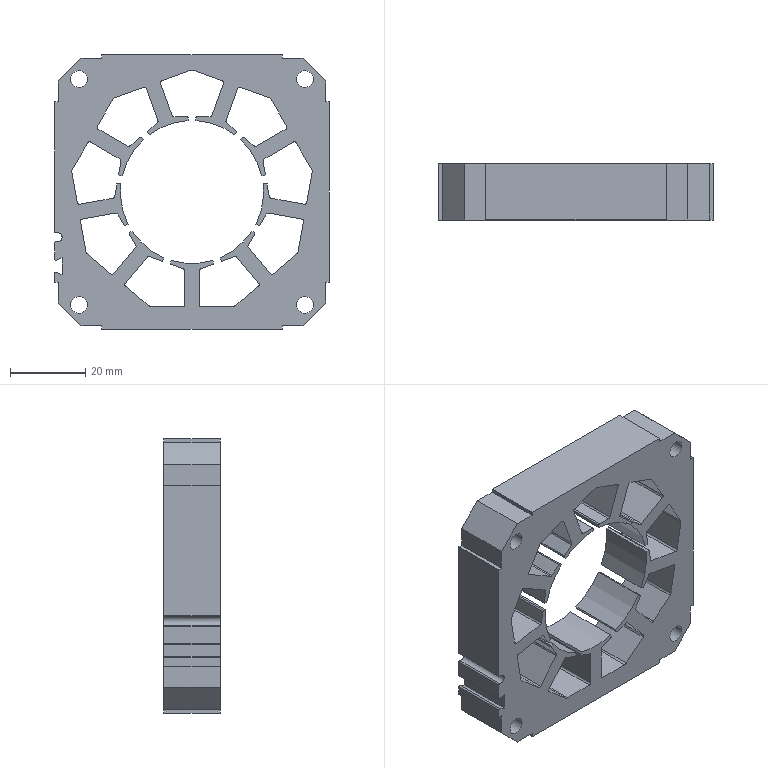Part | STEP file | DINGZITIEXING_8_1 | 1 solid | 188 faces | box 73 x 15 x 73 mm | volume 38126 mm3 | plane 103 | cylinder 85 | commonest cylinder face diameters 1 x36 0.6 x22 2 x9 38 x9 4.5 x8 2.5 x1